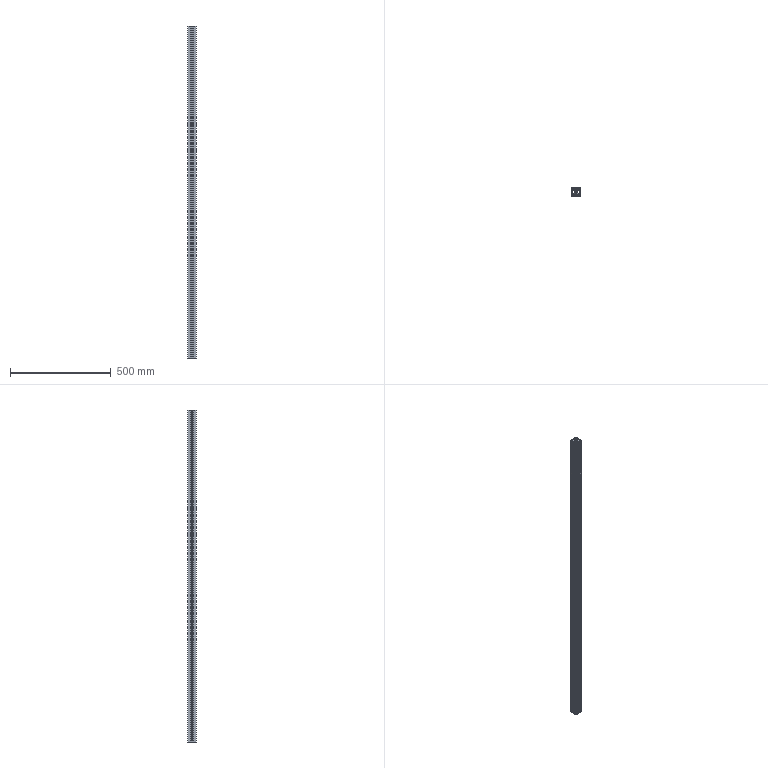Part | 1 solid | 196 faces | box 40 x 40 x 1650 mm | volume 682886 mm3 | plane 114 | cylinder 82 | commonest cylinder face diameters 2 x36 4 x16 10 x12 0.4 x8 6.8 x6 6.4 x4